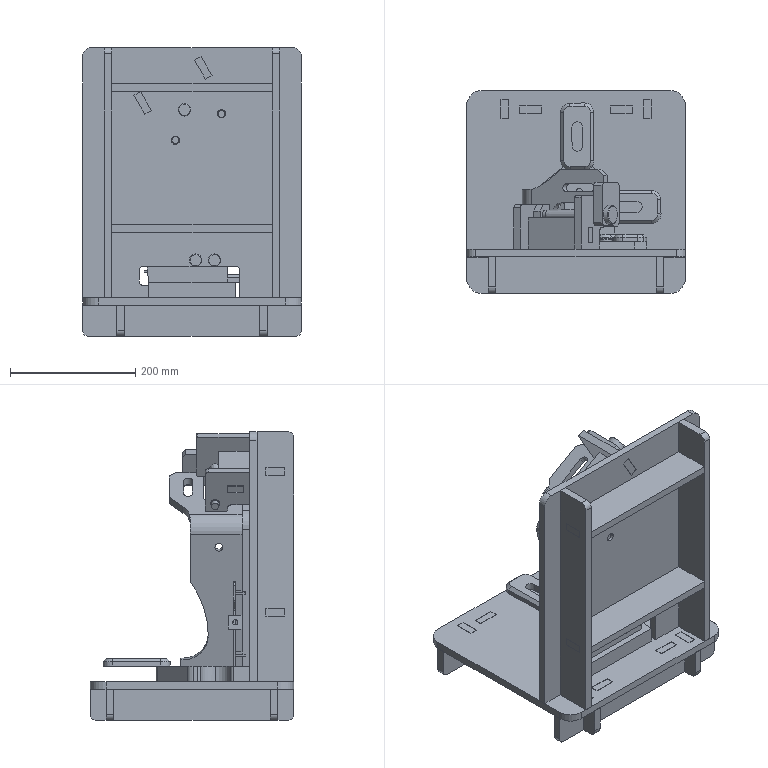Part | SolidWorks | features InContextFeatHolder 16, LocalLPattern 6, ReferencePattern 6, CosmeticWeldCutList 1 | 32 solids | 714 faces | box 350 x 325 x 462 mm | volume 6228356 mm3 | plane 499 | cylinder 156 | cone 58 | spline 1 | commonest cylinder face diameters 30 x26 20 x21 12.5 x20 10 x18 17 x18 13 x11